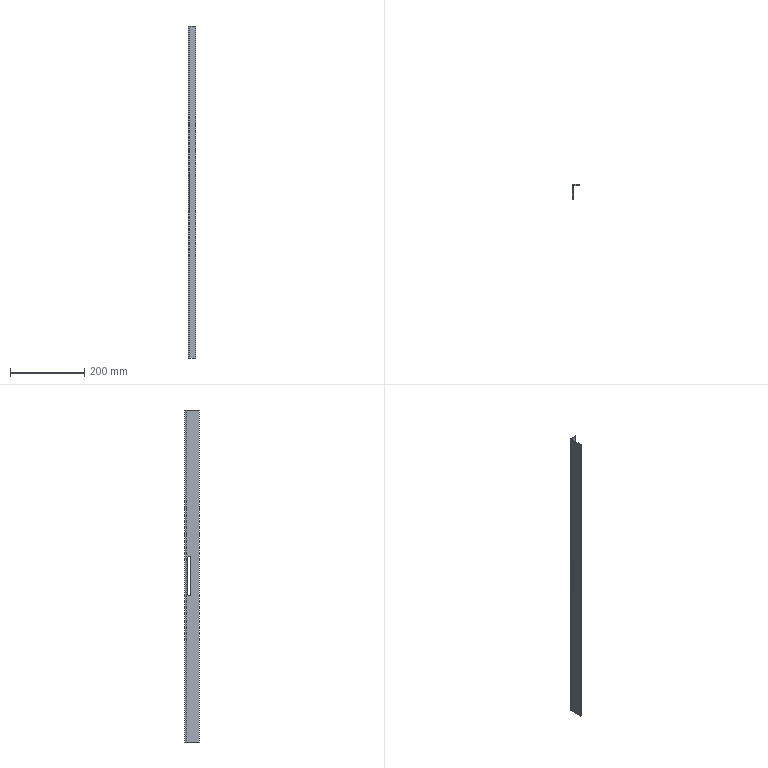Part | SolidWorks | features FlatPattern 1, ICE 1, SMBaseFlange 1, SheetMetal 1 | 1 solid | 19 faces | box 20 x 40 x 895 mm | volume 100259 mm3 | plane 14 | cylinder 5 | commonest cylinder face diameters 6 x3 4 x1 8 x1
STEP:
#1=CARTESIAN_POINT('',(0.,28.,394.5));
#2=VERTEX_POINT('',#1);
#3=CARTESIAN_POINT('',(0.,31.,397.5));
#4=VERTEX_POINT('',#3);
#5=CARTESIAN_POINT('',(0.,28.,397.5));
#6=DIRECTION('',(1.,0.,0.));
#7=DIRECTION('',(0.,0.,-1.));
#8=AXIS2_PLACEMENT_3D('',#5,#6,#7);
#9=CIRCLE('',#8,3.);
#10=EDGE_CURVE('',#2,#4,#9,.T.);
#11=ORIENTED_EDGE('',*,*,#10,.F.);
#12=CARTESIAN_POINT('',(2.,28.,394.5));
#13=VERTEX_POINT('',#12);
#14=CARTESIAN_POINT('',(0.,28.,394.5));
#15=DIRECTION('',(1.,0.,0.));
#16=VECTOR('',#15,1000.);
#17=LINE('',#14,#16);
#18=EDGE_CURVE('',#2,#13,#17,.T.);
#19=ORIENTED_EDGE('',*,*,#18,.T.);
#20=CARTESIAN_POINT('',(2.,31.,397.5));
#21=VERTEX_POINT('',#20);
#22=CARTESIAN_POINT('',(2.,28.,397.5));
#23=DIRECTION('',(1.,0.,0.));
#24=DIRECTION('',(0.,0.,-1.));
#25=AXIS2_PLACEMENT_3D('',#22,#23,#24);
#26=CIRCLE('',#25,3.);
#27=EDGE_CURVE('',#13,#21,#26,.T.);
#28=ORIENTED_EDGE('',*,*,#27,.T.);
#29=CARTESIAN_POINT('',(0.,31.,397.5));
#30=DIRECTION('',(1.,0.,0.));
#31=VECTOR('',#30,1000.);
#32=LINE('',#29,#31);
#33=EDGE_CURVE('',#4,#21,#32,.T.);
#34=ORIENTED_EDGE('',*,*,#33,.F.);
#35=EDGE_LOOP('',(#11,#19,#28,#34));
#36=FACE_OUTER_BOUND('',#35,.T.);
#37=CARTESIAN_POINT('',(0.,28.,397.5));
#38=DIRECTION('',(1.,0.,0.));
#39=DIRECTION('',(0.,0.,-1.));
#40=AXIS2_PLACEMENT_3D('',#37,#38,#39);
#41=CYLINDRICAL_SURFACE('',#40,3.);
#42=ADVANCED_FACE('',(#36),#41,.F.);
#43=CARTESIAN_POINT('',(4.,40.,895.));
#44=VERTEX_POINT('',#43);
#45=CARTESIAN_POINT('',(4.,38.,895.));
#46=VERTEX_POINT('',#45);
#47=CARTESIAN_POINT('',(4.,40.,895.));
#48=DIRECTION('',(0.,-1.,0.));
#49=VECTOR('',#48,1000.);
#50=LINE('',#47,#49);
#51=EDGE_CURVE('',#44,#46,#50,.T.);
#52=ORIENTED_EDGE('',*,*,#51,.F.);
#53=CARTESIAN_POINT('',(0.,36.,895.));
#54=VERTEX_POINT('',#53);
#55=CARTESIAN_POINT('',(4.,36.,895.));
#56=DIRECTION('',(0.,0.,-1.));
#57=DIRECTION('',(1.,0.,0.));
#58=AXIS2_PLACEMENT_3D('',#55,#56,#57);
#59=CIRCLE('',#58,4.);
#60=EDGE_CURVE('',#54,#44,#59,.T.);
#61=ORIENTED_EDGE('',*,*,#60,.F.);
#62=CARTESIAN_POINT('',(2.,36.,895.));
#63=VERTEX_POINT('',#62);
#64=CARTESIAN_POINT('',(2.,36.,895.));
#65=DIRECTION('',(-1.,0.,0.));
#66=VECTOR('',#65,1000.);
#67=LINE('',#64,#66);
#68=EDGE_CURVE('',#63,#54,#67,.T.);
#69=ORIENTED_EDGE('',*,*,#68,.F.);
#70=CARTESIAN_POINT('',(4.,36.,895.));
#71=DIRECTION('',(0.,0.,-1.));
#72=DIRECTION('',(1.,0.,0.));
#73=AXIS2_PLACEMENT_3D('',#70,#71,#72);
#74=CIRCLE('',#73,2.);
#75=EDGE_CURVE('',#63,#46,#74,.T.);
#76=ORIENTED_EDGE('',*,*,#75,.T.);
#77=EDGE_LOOP('',(#52,#61,#69,#76));
#78=FACE_OUTER_BOUND('',#77,.T.);
#79=CARTESIAN_POINT('',(4.,40.,895.));
#80=DIRECTION('',(0.,0.,1.));
#81=DIRECTION('',(1.,0.,0.));
#82=AXIS2_PLACEMENT_3D('',#79,#80,#81);
#83=PLANE('',#82);
#84=ADVANCED_FACE('',(#78),#83,.T.);
#85=CARTESIAN_POINT('',(20.,40.,895.));
#86=VERTEX_POINT('',#85);
#87=CARTESIAN_POINT('',(0.,40.,895.));
#88=DIRECTION('',(1.,0.,0.));
#89=VECTOR('',#88,1000.);
#90=LINE('',#87,#89);
#91=EDGE_CURVE('',#44,#86,#90,.T.);
#92=ORIENTED_EDGE('',*,*,#91,.F.);
#93=ORIENTED_EDGE('',*,*,#51,.T.);
#94=CARTESIAN_POINT('',(20.,38.,895.));
#95=VERTEX_POINT('',#94);
#96=CARTESIAN_POINT('',(0.,38.,895.));
#97=DIRECTION('',(1.,0.,0.));
#98=VECTOR('',#97,1000.);
#99=LINE('',#96,#98);
#100=EDGE_CURVE('',#46,#95,#99,.T.);
#101=ORIENTED_EDGE('',*,*,#100,.T.);
#102=CARTESIAN_POINT('',(20.,40.,895.));
#103=DIRECTION('',(0.,-1.,0.));
#104=VECTOR('',#103,1000.);
#105=LINE('',#102,#104);
#106=EDGE_CURVE('',#86,#95,#105,.T.);
#107=ORIENTED_EDGE('',*,*,#106,.F.);
#108=EDGE_LOOP('',(#92,#93,#101,#107));
#109=FACE_OUTER_BOUND('',#108,.T.);
#110=CARTESIAN_POINT('',(2.,36.,895.));
#111=DIRECTION('',(0.,0.,1.));
#112=DIRECTION('',(1.,0.,0.));
#113=AXIS2_PLACEMENT_3D('',#110,#111,#112);
#114=PLANE('',#113);
#115=ADVANCED_FACE('',(#109),#114,.T.);
#116=CARTESIAN_POINT('',(0.,36.,0.));
#117=VERTEX_POINT('',#116);
#118=CARTESIAN_POINT('',(2.,36.,0.));
#119=VERTEX_POINT('',#118);
#120=CARTESIAN_POINT('',(0.,36.,0.));
#121=DIRECTION('',(1.,0.,0.));
#122=VECTOR('',#121,1000.);
#123=LINE('',#120,#122);
#124=EDGE_CURVE('',#117,#119,#123,.T.);
#125=ORIENTED_EDGE('',*,*,#124,.F.);
#126=CARTESIAN_POINT('',(4.,40.,0.));
#127=VERTEX_POINT('',#126);
#128=CARTESIAN_POINT('',(4.,36.,0.));
#129=DIRECTION('',(0.,0.,-1.));
#130=DIRECTION('',(1.,0.,0.));
#131=AXIS2_PLACEMENT_3D('',#128,#129,#130);
#132=CIRCLE('',#131,4.);
#133=EDGE_CURVE('',#117,#127,#132,.T.);
#134=ORIENTED_EDGE('',*,*,#133,.T.);
#135=CARTESIAN_POINT('',(4.,38.,0.));
#136=VERTEX_POINT('',#135);
#137=CARTESIAN_POINT('',(4.,38.,0.));
#138=DIRECTION('',(0.,1.,0.));
#139=VECTOR('',#138,1000.);
#140=LINE('',#137,#139);
#141=EDGE_CURVE('',#136,#127,#140,.T.);
#142=ORIENTED_EDGE('',*,*,#141,.F.);
#143=CARTESIAN_POINT('',(4.,36.,0.));
#144=DIRECTION('',(0.,0.,-1.));
#145=DIRECTION('',(1.,0.,0.));
#146=AXIS2_PLACEMENT_3D('',#143,#144,#145);
#147=CIRCLE('',#146,2.);
#148=EDGE_CURVE('',#119,#136,#147,.T.);
#149=ORIENTED_EDGE('',*,*,#148,.F.);
#150=EDGE_LOOP('',(#125,#134,#142,#149));
#151=FACE_OUTER_BOUND('',#150,.T.);
#152=CARTESIAN_POINT('',(0.,36.,0.));
#153=DIRECTION('',(0.,0.,-1.));
#154=DIRECTION('',(-1.,0.,0.));
#155=AXIS2_PLACEMENT_3D('',#152,#153,#154);
#156=PLANE('',#155);
#157=ADVANCED_FACE('',(#151),#156,.T.);
#158=CARTESIAN_POINT('',(0.,0.,0.));
#159=VERTEX_POINT('',#158);
#160=CARTESIAN_POINT('',(0.,0.,0.));
#161=DIRECTION('',(0.,1.,0.));
#162=VECTOR('',#161,1000.);
#163=LINE('',#160,#162);
#164=EDGE_CURVE('',#159,#117,#163,.T.);
#165=ORIENTED_EDGE('',*,*,#164,.T.);
#166=ORIENTED_EDGE('',*,*,#124,.T.);
#167=CARTESIAN_POINT('',(2.,0.,0.));
#168=VERTEX_POINT('',#167);
#169=CARTESIAN_POINT('',(2.,0.,0.));
#170=DIRECTION('',(0.,1.,0.));
#171=VECTOR('',#170,1000.);
#172=LINE('',#169,#171);
#173=EDGE_CURVE('',#168,#119,#172,.T.);
#174=ORIENTED_EDGE('',*,*,#173,.F.);
#175=CARTESIAN_POINT('',(2.,0.,0.));
#176=DIRECTION('',(-1.,0.,0.));
#177=VECTOR('',#176,1000.);
#178=LINE('',#175,#177);
#179=EDGE_CURVE('',#168,#159,#178,.T.);
#180=ORIENTED_EDGE('',*,*,#179,.T.);
#181=EDGE_LOOP('',(#165,#166,#174,#180));
#182=FACE_OUTER_BOUND('',#181,.T.);
#183=CARTESIAN_POINT('',(4.,38.,0.));
#184=DIRECTION('',(0.,0.,-1.));
#185=DIRECTION('',(-1.,0.,0.));
#186=AXIS2_PLACEMENT_3D('',#183,#184,#185);
#187=PLANE('',#186);
#188=ADVANCED_FACE('',(#182),#187,.T.);
#189=CARTESIAN_POINT('',(20.,38.,0.));
#190=VERTEX_POINT('',#189);
#191=CARTESIAN_POINT('',(0.,38.,0.));
#192=DIRECTION('',(1.,0.,0.));
#193=VECTOR('',#192,1000.);
#194=LINE('',#191,#193);
#195=EDGE_CURVE('',#136,#190,#194,.T.);
#196=ORIENTED_EDGE('',*,*,#195,.T.);
#197=CARTESIAN_POINT('',(20.,38.,895.));
#198=DIRECTION('',(0.,0.,-1.));
#199=VECTOR('',#198,1000.);
#200=LINE('',#197,#199);
#201=EDGE_CURVE('',#95,#190,#200,.T.);
#202=ORIENTED_EDGE('',*,*,#201,.F.);
#203=ORIENTED_EDGE('',*,*,#100,.F.);
#204=CARTESIAN_POINT('',(4.,38.,895.));
#205=DIRECTION('',(0.,0.,-1.));
#206=VECTOR('',#205,1000.);
#207=LINE('',#204,#206);
#208=EDGE_CURVE('',#46,#136,#207,.T.);
#209=ORIENTED_EDGE('',*,*,#208,.T.);
#210=EDGE_LOOP('',(#196,#202,#203,#209));
#211=FACE_OUTER_BOUND('',#210,.T.);
#212=CARTESIAN_POINT('',(0.,38.,895.));
#213=DIRECTION('',(0.,1.,0.));
#214=DIRECTION('',(0.,0.,1.));
#215=AXIS2_PLACEMENT_3D('',#212,#213,#214);
#216=PLANE('',#215);
#217=ADVANCED_FACE('',(#211),#216,.F.);
#218=CARTESIAN_POINT('',(20.,40.,0.));
#219=VERTEX_POINT('',#218);
#220=CARTESIAN_POINT('',(20.,40.,0.));
#221=DIRECTION('',(0.,-1.,0.));
#222=VECTOR('',#221,1000.);
#223=LINE('',#220,#222);
#224=EDGE_CURVE('',#219,#190,#223,.T.);
#225=ORIENTED_EDGE('',*,*,#224,.F.);
#226=CARTESIAN_POINT('',(20.,40.,895.));
#227=DIRECTION('',(0.,0.,-1.));
#228=VECTOR('',#227,1000.);
#229=LINE('',#226,#228);
#230=EDGE_CURVE('',#86,#219,#229,.T.);
#231=ORIENTED_EDGE('',*,*,#230,.F.);
#232=ORIENTED_EDGE('',*,*,#106,.T.);
#233=ORIENTED_EDGE('',*,*,#201,.T.);
#234=EDGE_LOOP('',(#225,#231,#232,#233));
#235=FACE_OUTER_BOUND('',#234,.T.);
#236=CARTESIAN_POINT('',(20.,40.,895.));
#237=DIRECTION('',(1.,0.,0.));
#238=DIRECTION('',(0.,0.,-1.));
#239=AXIS2_PLACEMENT_3D('',#236,#237,#238);
#240=PLANE('',#239);
#241=ADVANCED_FACE('',(#235),#240,.T.);
#242=CARTESIAN_POINT('',(0.,40.,0.));
#243=DIRECTION('',(1.,0.,0.));
#244=VECTOR('',#243,1000.);
#245=LINE('',#242,#244);
#246=EDGE_CURVE('',#127,#219,#245,.T.);
#247=ORIENTED_EDGE('',*,*,#246,.F.);
#248=CARTESIAN_POINT('',(4.,40.,895.));
#249=DIRECTION('',(0.,0.,-1.));
#250=VECTOR('',#249,1000.);
#251=LINE('',#248,#250);
#252=EDGE_CURVE('',#44,#127,#251,.T.);
#253=ORIENTED_EDGE('',*,*,#252,.F.);
#254=ORIENTED_EDGE('',*,*,#91,.T.);
#255=ORIENTED_EDGE('',*,*,#230,.T.);
#256=EDGE_LOOP('',(#247,#253,#254,#255));
#257=FACE_OUTER_BOUND('',#256,.T.);
#258=CARTESIAN_POINT('',(0.,40.,895.));
#259=DIRECTION('',(0.,1.,0.));
#260=DIRECTION('',(0.,0.,1.));
#261=AXIS2_PLACEMENT_3D('',#258,#259,#260);
#262=PLANE('',#261);
#263=ADVANCED_FACE('',(#257),#262,.T.);
#264=ORIENTED_EDGE('',*,*,#133,.F.);
#265=CARTESIAN_POINT('',(0.,36.,895.));
#266=DIRECTION('',(0.,0.,-1.));
#267=VECTOR('',#266,1000.);
#268=LINE('',#265,#267);
#269=EDGE_CURVE('',#54,#117,#268,.T.);
#270=ORIENTED_EDGE('',*,*,#269,.F.);
#271=ORIENTED_EDGE('',*,*,#60,.T.);
#272=ORIENTED_EDGE('',*,*,#252,.T.);
#273=EDGE_LOOP('',(#264,#270,#271,#272));
#274=FACE_OUTER_BOUND('',#273,.T.);
#275=CARTESIAN_POINT('',(4.,36.,895.));
#276=DIRECTION('',(0.,0.,-1.));
#277=DIRECTION('',(-1.,0.,0.));
#278=AXIS2_PLACEMENT_3D('',#275,#276,#277);
#279=CYLINDRICAL_SURFACE('',#278,4.);
#280=ADVANCED_FACE('',(#274),#279,.T.);
#281=CARTESIAN_POINT('',(0.,25.,397.5));
#282=VERTEX_POINT('',#281);
#283=CARTESIAN_POINT('',(0.,28.,397.5));
#284=DIRECTION('',(1.,0.,0.));
#285=DIRECTION('',(0.,0.,-1.));
#286=AXIS2_PLACEMENT_3D('',#283,#284,#285);
#287=CIRCLE('',#286,3.);
#288=EDGE_CURVE('',#282,#2,#287,.T.);
#289=ORIENTED_EDGE('',*,*,#288,.T.);
#290=ORIENTED_EDGE('',*,*,#10,.T.);
#291=CARTESIAN_POINT('',(0.,31.,497.5));
#292=VERTEX_POINT('',#291);
#293=CARTESIAN_POINT('',(0.,31.,397.5));
#294=DIRECTION('',(0.,0.,1.));
#295=VECTOR('',#294,1000.);
#296=LINE('',#293,#295);
#297=EDGE_CURVE('',#4,#292,#296,.T.);
#298=ORIENTED_EDGE('',*,*,#297,.T.);
#299=CARTESIAN_POINT('',(0.,25.,497.5));
#300=VERTEX_POINT('',#299);
#301=CARTESIAN_POINT('',(0.,28.,497.5));
#302=DIRECTION('',(1.,0.,0.));
#303=DIRECTION('',(0.,0.,-1.));
#304=AXIS2_PLACEMENT_3D('',#301,#302,#303);
#305=CIRCLE('',#304,3.);
#306=EDGE_CURVE('',#292,#300,#305,.T.);
#307=ORIENTED_EDGE('',*,*,#306,.T.);
#308=CARTESIAN_POINT('',(0.,25.,397.5));
#309=DIRECTION('',(0.,0.,-1.));
#310=VECTOR('',#309,1000.);
#311=LINE('',#308,#310);
#312=EDGE_CURVE('',#300,#282,#311,.T.);
#313=ORIENTED_EDGE('',*,*,#312,.T.);
#314=EDGE_LOOP('',(#289,#290,#298,#307,#313));
#315=FACE_BOUND('',#314,.T.);
#316=ORIENTED_EDGE('',*,*,#164,.F.);
#317=CARTESIAN_POINT('',(0.,0.,895.));
#318=VERTEX_POINT('',#317);
#319=CARTESIAN_POINT('',(0.,0.,895.));
#320=DIRECTION('',(0.,0.,-1.));
#321=VECTOR('',#320,1000.);
#322=LINE('',#319,#321);
#323=EDGE_CURVE('',#318,#159,#322,.T.);
#324=ORIENTED_EDGE('',*,*,#323,.F.);
#325=CARTESIAN_POINT('',(0.,0.,895.));
#326=DIRECTION('',(0.,1.,0.));
#327=VECTOR('',#326,1000.);
#328=LINE('',#325,#327);
#329=EDGE_CURVE('',#318,#54,#328,.T.);
#330=ORIENTED_EDGE('',*,*,#329,.T.);
#331=ORIENTED_EDGE('',*,*,#269,.T.);
#332=EDGE_LOOP('',(#316,#324,#330,#331));
#333=FACE_OUTER_BOUND('',#332,.T.);
#334=CARTESIAN_POINT('',(0.,0.,895.));
#335=DIRECTION('',(-1.,0.,0.));
#336=DIRECTION('',(0.,0.,1.));
#337=AXIS2_PLACEMENT_3D('',#334,#335,#336);
#338=PLANE('',#337);
#339=ADVANCED_FACE('',(#315,#333),#338,.T.);
#340=ORIENTED_EDGE('',*,*,#179,.F.);
#341=CARTESIAN_POINT('',(2.,0.,895.));
#342=VERTEX_POINT('',#341);
#343=CARTESIAN_POINT('',(2.,0.,895.));
#344=DIRECTION('',(0.,0.,-1.));
#345=VECTOR('',#344,1000.);
#346=LINE('',#343,#345);
#347=EDGE_CURVE('',#342,#168,#346,.T.);
#348=ORIENTED_EDGE('',*,*,#347,.F.);
#349=CARTESIAN_POINT('',(2.,0.,895.));
#350=DIRECTION('',(-1.,0.,0.));
#351=VECTOR('',#350,1000.);
#352=LINE('',#349,#351);
#353=EDGE_CURVE('',#342,#318,#352,.T.);
#354=ORIENTED_EDGE('',*,*,#353,.T.);
#355=ORIENTED_EDGE('',*,*,#323,.T.);
#356=EDGE_LOOP('',(#340,#348,#354,#355));
#357=FACE_OUTER_BOUND('',#356,.T.);
#358=CARTESIAN_POINT('',(2.,0.,895.));
#359=DIRECTION('',(0.,-1.,0.));
#360=DIRECTION('',(0.,0.,-1.));
#361=AXIS2_PLACEMENT_3D('',#358,#359,#360);
#362=PLANE('',#361);
#363=ADVANCED_FACE('',(#357),#362,.T.);
#364=CARTESIAN_POINT('',(2.,31.,497.5));
#365=VERTEX_POINT('',#364);
#366=CARTESIAN_POINT('',(2.,31.,397.5));
#367=DIRECTION('',(0.,0.,1.));
#368=VECTOR('',#367,1000.);
#369=LINE('',#366,#368);
#370=EDGE_CURVE('',#21,#365,#369,.T.);
#371=ORIENTED_EDGE('',*,*,#370,.F.);
#372=ORIENTED_EDGE('',*,*,#27,.F.);
#373=CARTESIAN_POINT('',(2.,25.,397.5));
#374=VERTEX_POINT('',#373);
#375=CARTESIAN_POINT('',(2.,28.,397.5));
#376=DIRECTION('',(1.,0.,0.));
#377=DIRECTION('',(0.,0.,-1.));
#378=AXIS2_PLACEMENT_3D('',#375,#376,#377);
#379=CIRCLE('',#378,3.);
#380=EDGE_CURVE('',#374,#13,#379,.T.);
#381=ORIENTED_EDGE('',*,*,#380,.F.);
#382=CARTESIAN_POINT('',(2.,25.,497.5));
#383=VERTEX_POINT('',#382);
#384=CARTESIAN_POINT('',(2.,25.,397.5));
#385=DIRECTION('',(0.,0.,-1.));
#386=VECTOR('',#385,1000.);
#387=LINE('',#384,#386);
#388=EDGE_CURVE('',#383,#374,#387,.T.);
#389=ORIENTED_EDGE('',*,*,#388,.F.);
#390=CARTESIAN_POINT('',(2.,28.,497.5));
#391=DIRECTION('',(1.,0.,0.));
#392=DIRECTION('',(0.,0.,-1.));
#393=AXIS2_PLACEMENT_3D('',#390,#391,#392);
#394=CIRCLE('',#393,3.);
#395=EDGE_CURVE('',#365,#383,#394,.T.);
#396=ORIENTED_EDGE('',*,*,#395,.F.);
#397=EDGE_LOOP('',(#371,#372,#381,#389,#396));
#398=FACE_BOUND('',#397,.T.);
#399=ORIENTED_EDGE('',*,*,#173,.T.);
#400=CARTESIAN_POINT('',(2.,36.,895.));
#401=DIRECTION('',(0.,0.,-1.));
#402=VECTOR('',#401,1000.);
#403=LINE('',#400,#402);
#404=EDGE_CURVE('',#63,#119,#403,.T.);
#405=ORIENTED_EDGE('',*,*,#404,.F.);
#406=CARTESIAN_POINT('',(2.,0.,895.));
#407=DIRECTION('',(0.,1.,0.));
#408=VECTOR('',#407,1000.);
#409=LINE('',#406,#408);
#410=EDGE_CURVE('',#342,#63,#409,.T.);
#411=ORIENTED_EDGE('',*,*,#410,.F.);
#412=ORIENTED_EDGE('',*,*,#347,.T.);
#413=EDGE_LOOP('',(#399,#405,#411,#412));
#414=FACE_OUTER_BOUND('',#413,.T.);
#415=CARTESIAN_POINT('',(2.,0.,895.));
#416=DIRECTION('',(-1.,0.,0.));
#417=DIRECTION('',(0.,0.,1.));
#418=AXIS2_PLACEMENT_3D('',#415,#416,#417);
#419=PLANE('',#418);
#420=ADVANCED_FACE('',(#398,#414),#419,.F.);
#421=ORIENTED_EDGE('',*,*,#148,.T.);
#422=ORIENTED_EDGE('',*,*,#208,.F.);
#423=ORIENTED_EDGE('',*,*,#75,.F.);
#424=ORIENTED_EDGE('',*,*,#404,.T.);
#425=EDGE_LOOP('',(#421,#422,#423,#424));
#426=FACE_OUTER_BOUND('',#425,.T.);
#427=CARTESIAN_POINT('',(4.,36.,895.));
#428=DIRECTION('',(0.,0.,-1.));
#429=DIRECTION('',(-1.,0.,0.));
#430=AXIS2_PLACEMENT_3D('',#427,#428,#429);
#431=CYLINDRICAL_SURFACE('',#430,2.);
#432=ADVANCED_FACE('',(#426),#431,.F.);
#433=ORIENTED_EDGE('',*,*,#410,.T.);
#434=ORIENTED_EDGE('',*,*,#68,.T.);
#435=ORIENTED_EDGE('',*,*,#329,.F.);
#436=ORIENTED_EDGE('',*,*,#353,.F.);
#437=EDGE_LOOP('',(#433,#434,#435,#436));
#438=FACE_OUTER_BOUND('',#437,.T.);
#439=CARTESIAN_POINT('',(4.,36.,895.));
#440=DIRECTION('',(0.,0.,1.));
#441=DIRECTION('',(1.,0.,0.));
#442=AXIS2_PLACEMENT_3D('',#439,#440,#441);
#443=PLANE('',#442);
#444=ADVANCED_FACE('',(#438),#443,.T.);
#445=ORIENTED_EDGE('',*,*,#195,.F.);
#446=ORIENTED_EDGE('',*,*,#141,.T.);
#447=ORIENTED_EDGE('',*,*,#246,.T.);
#448=ORIENTED_EDGE('',*,*,#224,.T.);
#449=EDGE_LOOP('',(#445,#446,#447,#448));
#450=FACE_OUTER_BOUND('',#449,.T.);
#451=CARTESIAN_POINT('',(4.,36.,0.));
#452=DIRECTION('',(0.,0.,1.));
#453=DIRECTION('',(1.,0.,0.));
#454=AXIS2_PLACEMENT_3D('',#451,#452,#453);
#455=PLANE('',#454);
#456=ADVANCED_FACE('',(#450),#455,.F.);
#457=ORIENTED_EDGE('',*,*,#18,.F.);
#458=ORIENTED_EDGE('',*,*,#288,.F.);
#459=CARTESIAN_POINT('',(0.,25.,397.5));
#460=DIRECTION('',(1.,0.,0.));
#461=VECTOR('',#460,1000.);
#462=LINE('',#459,#461);
#463=EDGE_CURVE('',#282,#374,#462,.T.);
#464=ORIENTED_EDGE('',*,*,#463,.T.);
#465=ORIENTED_EDGE('',*,*,#380,.T.);
#466=EDGE_LOOP('',(#457,#458,#464,#465));
#467=FACE_OUTER_BOUND('',#466,.T.);
#468=CARTESIAN_POINT('',(0.,28.,397.5));
#469=DIRECTION('',(1.,0.,0.));
#470=DIRECTION('',(0.,0.,-1.));
#471=AXIS2_PLACEMENT_3D('',#468,#469,#470);
#472=CYLINDRICAL_SURFACE('',#471,3.);
#473=ADVANCED_FACE('',(#467),#472,.F.);
#474=ORIENTED_EDGE('',*,*,#388,.T.);
#475=ORIENTED_EDGE('',*,*,#463,.F.);
#476=ORIENTED_EDGE('',*,*,#312,.F.);
#477=CARTESIAN_POINT('',(0.,25.,497.5));
#478=DIRECTION('',(1.,0.,0.));
#479=VECTOR('',#478,1000.);
#480=LINE('',#477,#479);
#481=EDGE_CURVE('',#300,#383,#480,.T.);
#482=ORIENTED_EDGE('',*,*,#481,.T.);
#483=EDGE_LOOP('',(#474,#475,#476,#482));
#484=FACE_OUTER_BOUND('',#483,.T.);
#485=CARTESIAN_POINT('',(0.,25.,397.5));
#486=DIRECTION('',(0.,-1.,0.));
#487=DIRECTION('',(0.,0.,-1.));
#488=AXIS2_PLACEMENT_3D('',#485,#486,#487);
#489=PLANE('',#488);
#490=ADVANCED_FACE('',(#484),#489,.F.);
#491=ORIENTED_EDGE('',*,*,#395,.T.);
#492=ORIENTED_EDGE('',*,*,#481,.F.);
#493=ORIENTED_EDGE('',*,*,#306,.F.);
#494=CARTESIAN_POINT('',(0.,31.,497.5));
#495=DIRECTION('',(1.,0.,0.));
#496=VECTOR('',#495,1000.);
#497=LINE('',#494,#496);
#498=EDGE_CURVE('',#292,#365,#497,.T.);
#499=ORIENTED_EDGE('',*,*,#498,.T.);
#500=EDGE_LOOP('',(#491,#492,#493,#499));
#501=FACE_OUTER_BOUND('',#500,.T.);
#502=CARTESIAN_POINT('',(0.,28.,497.5));
#503=DIRECTION('',(1.,0.,0.));
#504=DIRECTION('',(0.,0.,-1.));
#505=AXIS2_PLACEMENT_3D('',#502,#503,#504);
#506=CYLINDRICAL_SURFACE('',#505,3.);
#507=ADVANCED_FACE('',(#501),#506,.F.);
#508=ORIENTED_EDGE('',*,*,#370,.T.);
#509=ORIENTED_EDGE('',*,*,#498,.F.);
#510=ORIENTED_EDGE('',*,*,#297,.F.);
#511=ORIENTED_EDGE('',*,*,#33,.T.);
#512=EDGE_LOOP('',(#508,#509,#510,#511));
#513=FACE_OUTER_BOUND('',#512,.T.);
#514=CARTESIAN_POINT('',(0.,31.,397.5));
#515=DIRECTION('',(0.,1.,0.));
#516=DIRECTION('',(0.,0.,1.));
#517=AXIS2_PLACEMENT_3D('',#514,#515,#516);
#518=PLANE('',#517);
#519=ADVANCED_FACE('',(#513),#518,.F.);
#520=CLOSED_SHELL('',(#42,#84,#115,#157,#188,#217,#241,#263,#280,#339,#363,#420,#432,#444,#456,#473,#490,#507,#519));
#521=MANIFOLD_SOLID_BREP('',#520);
#522=CARTESIAN_POINT('',(0.,0.,0.));
#523=DIRECTION('',(0.,0.,1.));
#524=DIRECTION('',(1.,0.,0.));
#525=AXIS2_PLACEMENT_3D('',#522,#523,#524);
#526=(LENGTH_UNIT()NAMED_UNIT(*)SI_UNIT(.MILLI.,.METRE.));
#527=UNCERTAINTY_MEASURE_WITH_UNIT(LENGTH_MEASURE(0.00001),#526,'','');
#528=(NAMED_UNIT(*)PLANE_ANGLE_UNIT()SI_UNIT($,.RADIAN.));
#529=(NAMED_UNIT(*)SI_UNIT($,.STERADIAN.)SOLID_ANGLE_UNIT());
#530=(GEOMETRIC_REPRESENTATION_CONTEXT(3)GLOBAL_UNCERTAINTY_ASSIGNED_CONTEXT((#527))GLOBAL_UNIT_ASSIGNED_CONTEXT((#526,#528,#529))REPRESENTATION_CONTEXT('',''));
#531=ADVANCED_BREP_SHAPE_REPRESENTATION('',(#521,#525),#530);